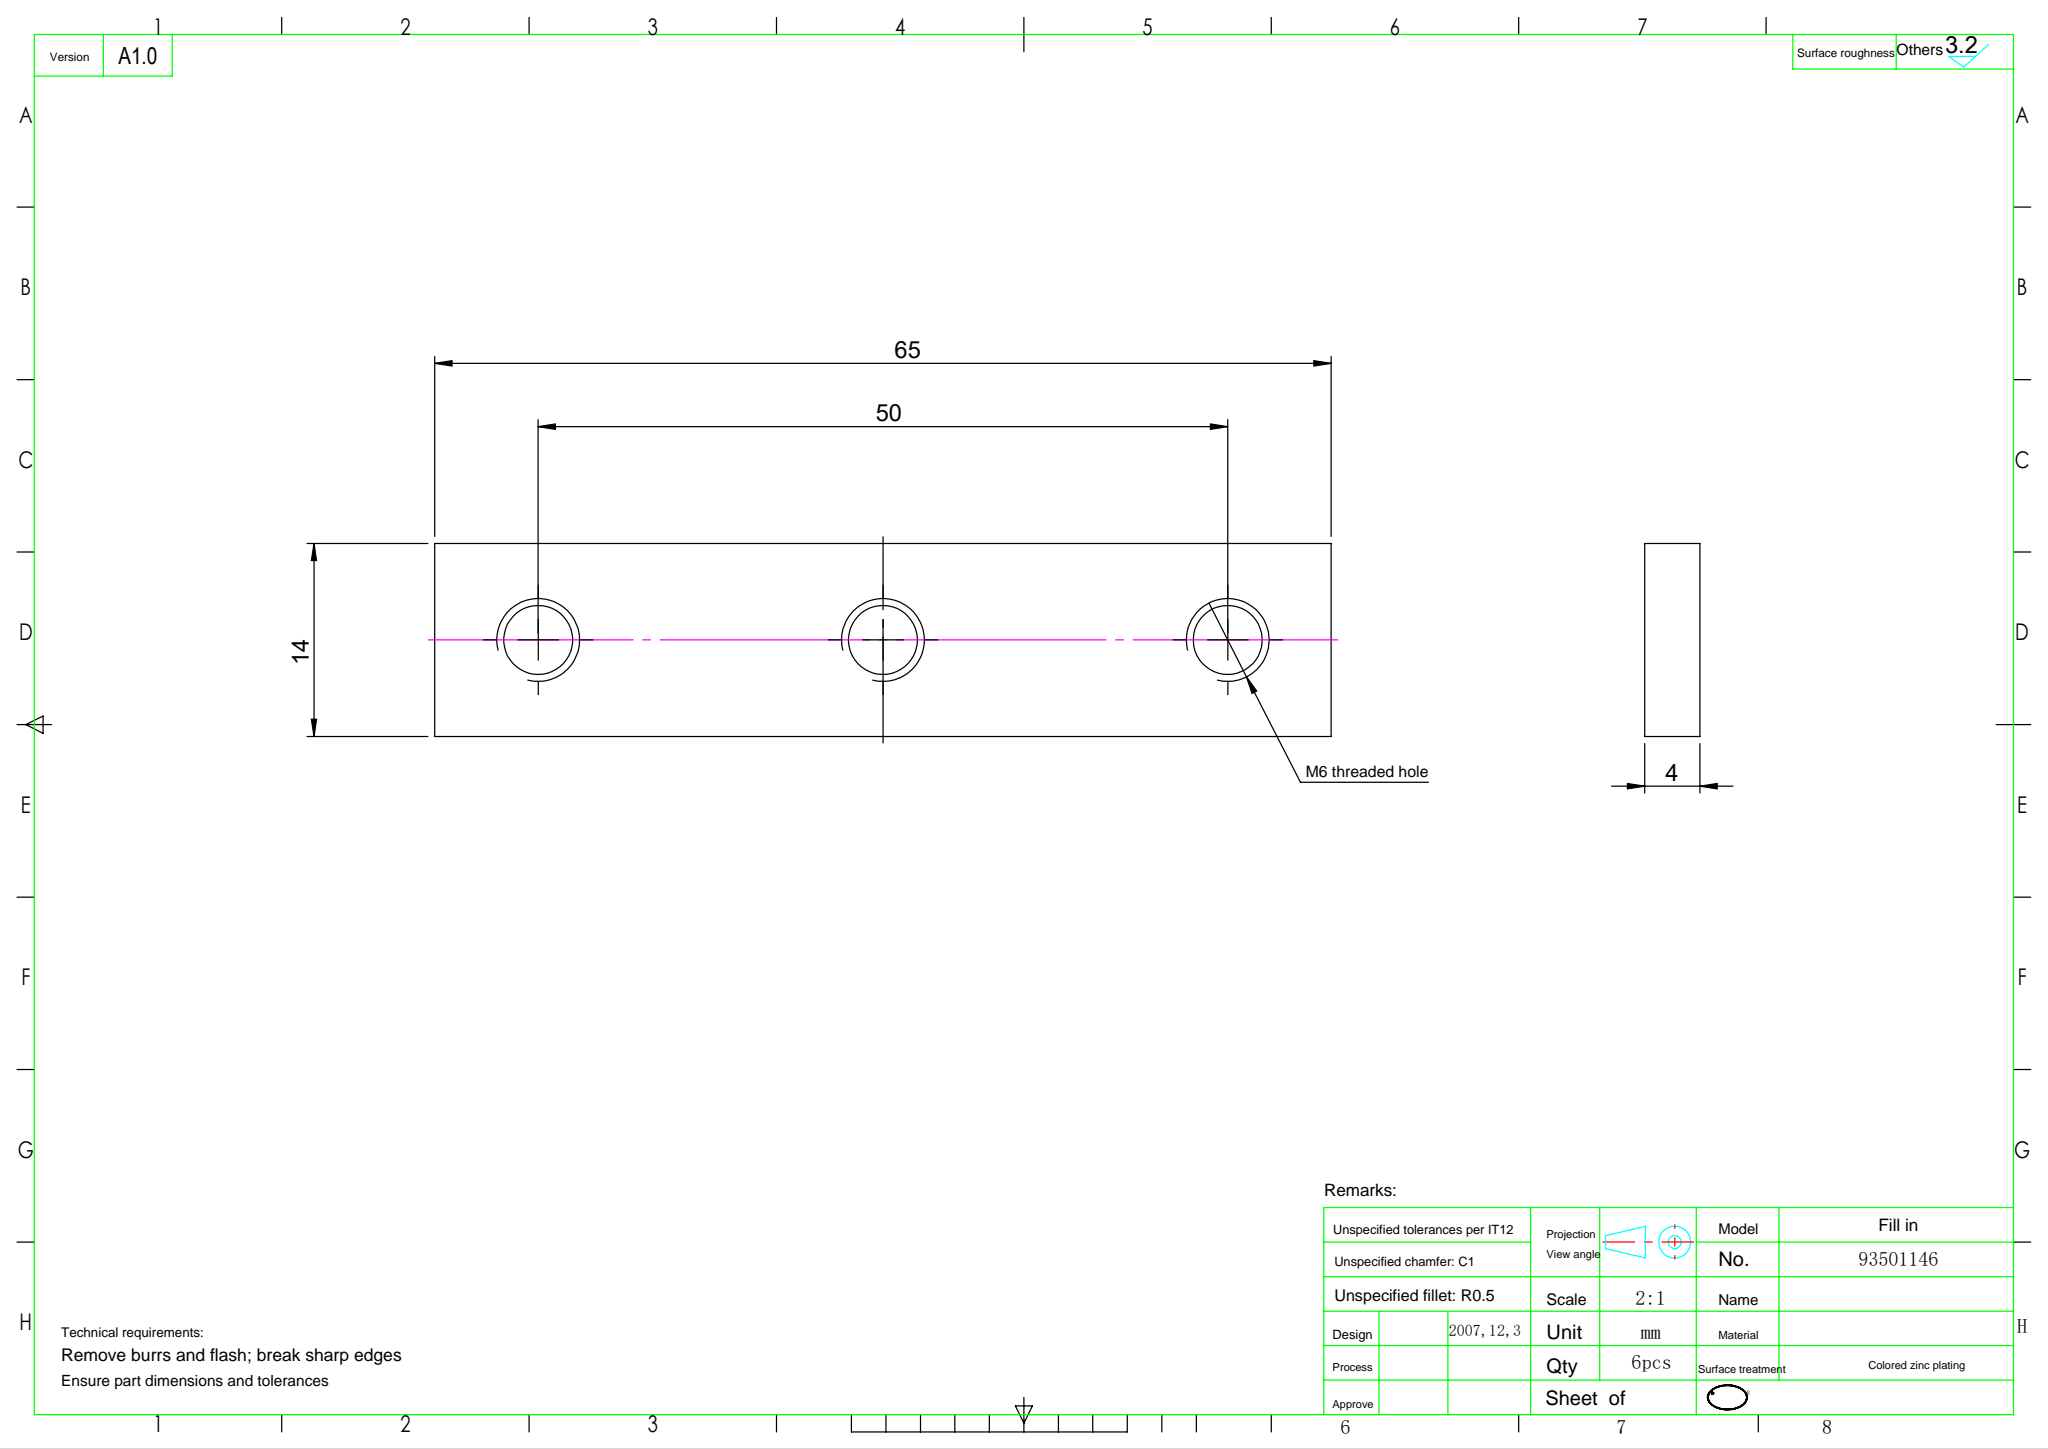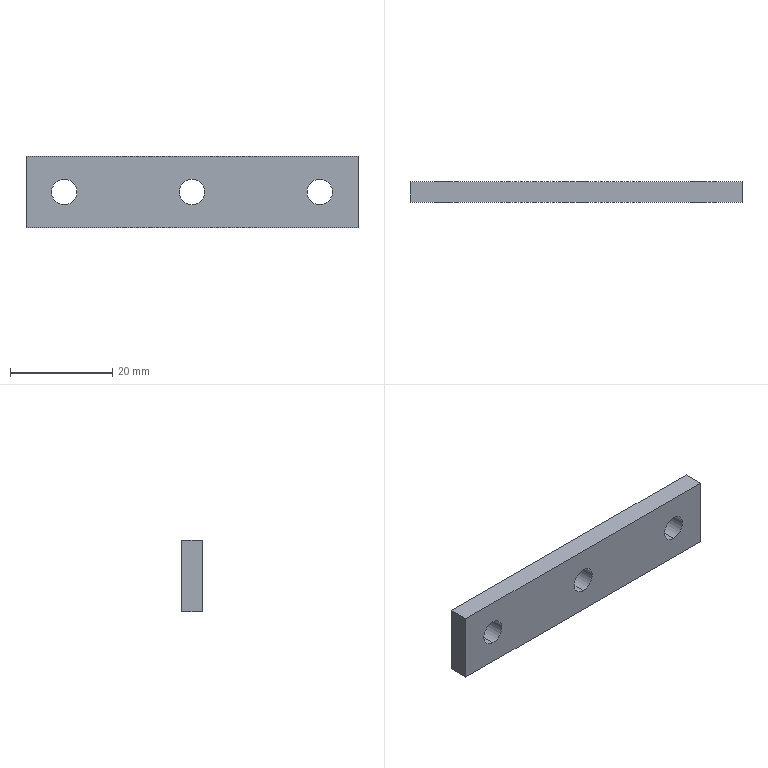Part | SolidWorks | features HoleWzd 1, ICE 1 | 1 solid | 12 faces | box 65 x 4 x 14 mm | volume 3404 mm3 | cylinder 6 | plane 6 | commonest cylinder face diameters 5 x6
STEP:
#1=CARTESIAN_POINT('',(-25.,-2.,-2.5));
#2=VERTEX_POINT('',#1);
#3=CARTESIAN_POINT('',(-25.,-2.,2.5));
#4=VERTEX_POINT('',#3);
#5=CARTESIAN_POINT('',(-25.,-2.,0.));
#6=DIRECTION('',(0.,1.,0.));
#7=DIRECTION('',(0.,0.,1.));
#8=AXIS2_PLACEMENT_3D('',#5,#6,#7);
#9=CIRCLE('',#8,2.5);
#10=EDGE_CURVE('',#2,#4,#9,.T.);
#11=ORIENTED_EDGE('',*,*,#10,.F.);
#12=CARTESIAN_POINT('',(-25.,2.,-2.5));
#13=VERTEX_POINT('',#12);
#14=CARTESIAN_POINT('',(-25.,2.,-2.5));
#15=DIRECTION('',(0.,1.,0.));
#16=VECTOR('',#15,1000.);
#17=LINE('',#14,#16);
#18=EDGE_CURVE('',#2,#13,#17,.T.);
#19=ORIENTED_EDGE('',*,*,#18,.T.);
#20=CARTESIAN_POINT('',(-25.,2.,2.5));
#21=VERTEX_POINT('',#20);
#22=CARTESIAN_POINT('',(-25.,2.,0.));
#23=DIRECTION('',(0.,1.,0.));
#24=DIRECTION('',(0.,0.,1.));
#25=AXIS2_PLACEMENT_3D('',#22,#23,#24);
#26=CIRCLE('',#25,2.5);
#27=EDGE_CURVE('',#13,#21,#26,.T.);
#28=ORIENTED_EDGE('',*,*,#27,.T.);
#29=CARTESIAN_POINT('',(-25.,2.,2.5));
#30=DIRECTION('',(0.,1.,0.));
#31=VECTOR('',#30,1000.);
#32=LINE('',#29,#31);
#33=EDGE_CURVE('',#4,#21,#32,.T.);
#34=ORIENTED_EDGE('',*,*,#33,.F.);
#35=EDGE_LOOP('',(#11,#19,#28,#34));
#36=FACE_OUTER_BOUND('',#35,.T.);
#37=CARTESIAN_POINT('',(-25.,2.,0.));
#38=DIRECTION('',(0.,1.,0.));
#39=DIRECTION('',(0.,0.,1.));
#40=AXIS2_PLACEMENT_3D('',#37,#38,#39);
#41=CYLINDRICAL_SURFACE('',#40,2.5);
#42=ADVANCED_FACE('',(#36),#41,.F.);
#43=CARTESIAN_POINT('',(0.,-2.,-2.5));
#44=VERTEX_POINT('',#43);
#45=CARTESIAN_POINT('',(0.,-2.,2.5));
#46=VERTEX_POINT('',#45);
#47=CARTESIAN_POINT('',(0.,-2.,0.));
#48=DIRECTION('',(0.,1.,0.));
#49=DIRECTION('',(0.,0.,1.));
#50=AXIS2_PLACEMENT_3D('',#47,#48,#49);
#51=CIRCLE('',#50,2.5);
#52=EDGE_CURVE('',#44,#46,#51,.T.);
#53=ORIENTED_EDGE('',*,*,#52,.F.);
#54=CARTESIAN_POINT('',(0.,2.,-2.5));
#55=VERTEX_POINT('',#54);
#56=CARTESIAN_POINT('',(0.,2.,-2.5));
#57=DIRECTION('',(0.,1.,0.));
#58=VECTOR('',#57,1000.);
#59=LINE('',#56,#58);
#60=EDGE_CURVE('',#44,#55,#59,.T.);
#61=ORIENTED_EDGE('',*,*,#60,.T.);
#62=CARTESIAN_POINT('',(0.,2.,2.5));
#63=VERTEX_POINT('',#62);
#64=CARTESIAN_POINT('',(0.,2.,0.));
#65=DIRECTION('',(0.,1.,0.));
#66=DIRECTION('',(0.,0.,1.));
#67=AXIS2_PLACEMENT_3D('',#64,#65,#66);
#68=CIRCLE('',#67,2.5);
#69=EDGE_CURVE('',#55,#63,#68,.T.);
#70=ORIENTED_EDGE('',*,*,#69,.T.);
#71=CARTESIAN_POINT('',(0.,2.,2.5));
#72=DIRECTION('',(0.,1.,0.));
#73=VECTOR('',#72,1000.);
#74=LINE('',#71,#73);
#75=EDGE_CURVE('',#46,#63,#74,.T.);
#76=ORIENTED_EDGE('',*,*,#75,.F.);
#77=EDGE_LOOP('',(#53,#61,#70,#76));
#78=FACE_OUTER_BOUND('',#77,.T.);
#79=CARTESIAN_POINT('',(0.,2.,0.));
#80=DIRECTION('',(0.,1.,0.));
#81=DIRECTION('',(0.,0.,1.));
#82=AXIS2_PLACEMENT_3D('',#79,#80,#81);
#83=CYLINDRICAL_SURFACE('',#82,2.5);
#84=ADVANCED_FACE('',(#78),#83,.F.);
#85=CARTESIAN_POINT('',(25.,-2.,-2.5));
#86=VERTEX_POINT('',#85);
#87=CARTESIAN_POINT('',(25.,-2.,2.5));
#88=VERTEX_POINT('',#87);
#89=CARTESIAN_POINT('',(25.,-2.,0.));
#90=DIRECTION('',(0.,1.,0.));
#91=DIRECTION('',(0.,0.,1.));
#92=AXIS2_PLACEMENT_3D('',#89,#90,#91);
#93=CIRCLE('',#92,2.5);
#94=EDGE_CURVE('',#86,#88,#93,.T.);
#95=ORIENTED_EDGE('',*,*,#94,.F.);
#96=CARTESIAN_POINT('',(25.,2.,-2.5));
#97=VERTEX_POINT('',#96);
#98=CARTESIAN_POINT('',(25.,2.,-2.5));
#99=DIRECTION('',(0.,1.,0.));
#100=VECTOR('',#99,1000.);
#101=LINE('',#98,#100);
#102=EDGE_CURVE('',#86,#97,#101,.T.);
#103=ORIENTED_EDGE('',*,*,#102,.T.);
#104=CARTESIAN_POINT('',(25.,2.,2.5));
#105=VERTEX_POINT('',#104);
#106=CARTESIAN_POINT('',(25.,2.,0.));
#107=DIRECTION('',(0.,1.,0.));
#108=DIRECTION('',(0.,0.,1.));
#109=AXIS2_PLACEMENT_3D('',#106,#107,#108);
#110=CIRCLE('',#109,2.5);
#111=EDGE_CURVE('',#97,#105,#110,.T.);
#112=ORIENTED_EDGE('',*,*,#111,.T.);
#113=CARTESIAN_POINT('',(25.,2.,2.5));
#114=DIRECTION('',(0.,1.,0.));
#115=VECTOR('',#114,1000.);
#116=LINE('',#113,#115);
#117=EDGE_CURVE('',#88,#105,#116,.T.);
#118=ORIENTED_EDGE('',*,*,#117,.F.);
#119=EDGE_LOOP('',(#95,#103,#112,#118));
#120=FACE_OUTER_BOUND('',#119,.T.);
#121=CARTESIAN_POINT('',(25.,2.,0.));
#122=DIRECTION('',(0.,1.,0.));
#123=DIRECTION('',(0.,0.,1.));
#124=AXIS2_PLACEMENT_3D('',#121,#122,#123);
#125=CYLINDRICAL_SURFACE('',#124,2.5);
#126=ADVANCED_FACE('',(#120),#125,.F.);
#127=CARTESIAN_POINT('',(32.5,-2.,7.));
#128=VERTEX_POINT('',#127);
#129=CARTESIAN_POINT('',(32.5,-2.,-7.));
#130=VERTEX_POINT('',#129);
#131=CARTESIAN_POINT('',(32.5,-2.,-7.));
#132=DIRECTION('',(0.,0.,-1.));
#133=VECTOR('',#132,1000.);
#134=LINE('',#131,#133);
#135=EDGE_CURVE('',#128,#130,#134,.T.);
#136=ORIENTED_EDGE('',*,*,#135,.T.);
#137=CARTESIAN_POINT('',(32.5,2.,-7.));
#138=VERTEX_POINT('',#137);
#139=CARTESIAN_POINT('',(32.5,2.,-7.));
#140=DIRECTION('',(0.,-1.,0.));
#141=VECTOR('',#140,1000.);
#142=LINE('',#139,#141);
#143=EDGE_CURVE('',#138,#130,#142,.T.);
#144=ORIENTED_EDGE('',*,*,#143,.F.);
#145=CARTESIAN_POINT('',(32.5,2.,7.));
#146=VERTEX_POINT('',#145);
#147=CARTESIAN_POINT('',(32.5,2.,-7.));
#148=DIRECTION('',(0.,0.,-1.));
#149=VECTOR('',#148,1000.);
#150=LINE('',#147,#149);
#151=EDGE_CURVE('',#146,#138,#150,.T.);
#152=ORIENTED_EDGE('',*,*,#151,.F.);
#153=CARTESIAN_POINT('',(32.5,2.,7.));
#154=DIRECTION('',(0.,-1.,0.));
#155=VECTOR('',#154,1000.);
#156=LINE('',#153,#155);
#157=EDGE_CURVE('',#146,#128,#156,.T.);
#158=ORIENTED_EDGE('',*,*,#157,.T.);
#159=EDGE_LOOP('',(#136,#144,#152,#158));
#160=FACE_OUTER_BOUND('',#159,.T.);
#161=CARTESIAN_POINT('',(32.5,2.,-7.));
#162=DIRECTION('',(-1.,0.,0.));
#163=DIRECTION('',(0.,0.,1.));
#164=AXIS2_PLACEMENT_3D('',#161,#162,#163);
#165=PLANE('',#164);
#166=ADVANCED_FACE('',(#160),#165,.F.);
#167=CARTESIAN_POINT('',(-32.5,-2.,-7.));
#168=VERTEX_POINT('',#167);
#169=CARTESIAN_POINT('',(-32.5,-2.,-7.));
#170=DIRECTION('',(-1.,0.,0.));
#171=VECTOR('',#170,1000.);
#172=LINE('',#169,#171);
#173=EDGE_CURVE('',#130,#168,#172,.T.);
#174=ORIENTED_EDGE('',*,*,#173,.T.);
#175=CARTESIAN_POINT('',(-32.5,2.,-7.));
#176=VERTEX_POINT('',#175);
#177=CARTESIAN_POINT('',(-32.5,2.,-7.));
#178=DIRECTION('',(0.,-1.,0.));
#179=VECTOR('',#178,1000.);
#180=LINE('',#177,#179);
#181=EDGE_CURVE('',#176,#168,#180,.T.);
#182=ORIENTED_EDGE('',*,*,#181,.F.);
#183=CARTESIAN_POINT('',(-32.5,2.,-7.));
#184=DIRECTION('',(-1.,0.,0.));
#185=VECTOR('',#184,1000.);
#186=LINE('',#183,#185);
#187=EDGE_CURVE('',#138,#176,#186,.T.);
#188=ORIENTED_EDGE('',*,*,#187,.F.);
#189=ORIENTED_EDGE('',*,*,#143,.T.);
#190=EDGE_LOOP('',(#174,#182,#188,#189));
#191=FACE_OUTER_BOUND('',#190,.T.);
#192=CARTESIAN_POINT('',(-32.5,2.,-7.));
#193=DIRECTION('',(0.,0.,1.));
#194=DIRECTION('',(1.,0.,0.));
#195=AXIS2_PLACEMENT_3D('',#192,#193,#194);
#196=PLANE('',#195);
#197=ADVANCED_FACE('',(#191),#196,.F.);
#198=CARTESIAN_POINT('',(-32.5,-2.,7.));
#199=VERTEX_POINT('',#198);
#200=CARTESIAN_POINT('',(-32.5,-2.,-7.));
#201=DIRECTION('',(0.,0.,1.));
#202=VECTOR('',#201,1000.);
#203=LINE('',#200,#202);
#204=EDGE_CURVE('',#168,#199,#203,.T.);
#205=ORIENTED_EDGE('',*,*,#204,.T.);
#206=CARTESIAN_POINT('',(-32.5,2.,7.));
#207=VERTEX_POINT('',#206);
#208=CARTESIAN_POINT('',(-32.5,2.,7.));
#209=DIRECTION('',(0.,-1.,0.));
#210=VECTOR('',#209,1000.);
#211=LINE('',#208,#210);
#212=EDGE_CURVE('',#207,#199,#211,.T.);
#213=ORIENTED_EDGE('',*,*,#212,.F.);
#214=CARTESIAN_POINT('',(-32.5,2.,-7.));
#215=DIRECTION('',(0.,0.,1.));
#216=VECTOR('',#215,1000.);
#217=LINE('',#214,#216);
#218=EDGE_CURVE('',#176,#207,#217,.T.);
#219=ORIENTED_EDGE('',*,*,#218,.F.);
#220=ORIENTED_EDGE('',*,*,#181,.T.);
#221=EDGE_LOOP('',(#205,#213,#219,#220));
#222=FACE_OUTER_BOUND('',#221,.T.);
#223=CARTESIAN_POINT('',(-32.5,2.,-7.));
#224=DIRECTION('',(1.,0.,0.));
#225=DIRECTION('',(0.,0.,-1.));
#226=AXIS2_PLACEMENT_3D('',#223,#224,#225);
#227=PLANE('',#226);
#228=ADVANCED_FACE('',(#222),#227,.F.);
#229=CARTESIAN_POINT('',(-32.5,-2.,7.));
#230=DIRECTION('',(1.,0.,0.));
#231=VECTOR('',#230,1000.);
#232=LINE('',#229,#231);
#233=EDGE_CURVE('',#199,#128,#232,.T.);
#234=ORIENTED_EDGE('',*,*,#233,.T.);
#235=ORIENTED_EDGE('',*,*,#157,.F.);
#236=CARTESIAN_POINT('',(-32.5,2.,7.));
#237=DIRECTION('',(1.,0.,0.));
#238=VECTOR('',#237,1000.);
#239=LINE('',#236,#238);
#240=EDGE_CURVE('',#207,#146,#239,.T.);
#241=ORIENTED_EDGE('',*,*,#240,.F.);
#242=ORIENTED_EDGE('',*,*,#212,.T.);
#243=EDGE_LOOP('',(#234,#235,#241,#242));
#244=FACE_OUTER_BOUND('',#243,.T.);
#245=CARTESIAN_POINT('',(-32.5,2.,7.));
#246=DIRECTION('',(0.,0.,-1.));
#247=DIRECTION('',(-1.,0.,0.));
#248=AXIS2_PLACEMENT_3D('',#245,#246,#247);
#249=PLANE('',#248);
#250=ADVANCED_FACE('',(#244),#249,.F.);
#251=CARTESIAN_POINT('',(-25.,2.,0.));
#252=DIRECTION('',(0.,1.,0.));
#253=DIRECTION('',(0.,0.,1.));
#254=AXIS2_PLACEMENT_3D('',#251,#252,#253);
#255=CIRCLE('',#254,2.5);
#256=EDGE_CURVE('',#21,#13,#255,.T.);
#257=ORIENTED_EDGE('',*,*,#256,.F.);
#258=ORIENTED_EDGE('',*,*,#27,.F.);
#259=EDGE_LOOP('',(#257,#258));
#260=FACE_BOUND('',#259,.T.);
#261=CARTESIAN_POINT('',(0.,2.,0.));
#262=DIRECTION('',(0.,1.,0.));
#263=DIRECTION('',(0.,0.,1.));
#264=AXIS2_PLACEMENT_3D('',#261,#262,#263);
#265=CIRCLE('',#264,2.5);
#266=EDGE_CURVE('',#63,#55,#265,.T.);
#267=ORIENTED_EDGE('',*,*,#266,.F.);
#268=ORIENTED_EDGE('',*,*,#69,.F.);
#269=EDGE_LOOP('',(#267,#268));
#270=FACE_BOUND('',#269,.T.);
#271=CARTESIAN_POINT('',(25.,2.,0.));
#272=DIRECTION('',(0.,1.,0.));
#273=DIRECTION('',(0.,0.,1.));
#274=AXIS2_PLACEMENT_3D('',#271,#272,#273);
#275=CIRCLE('',#274,2.5);
#276=EDGE_CURVE('',#105,#97,#275,.T.);
#277=ORIENTED_EDGE('',*,*,#276,.F.);
#278=ORIENTED_EDGE('',*,*,#111,.F.);
#279=EDGE_LOOP('',(#277,#278));
#280=FACE_BOUND('',#279,.T.);
#281=ORIENTED_EDGE('',*,*,#151,.T.);
#282=ORIENTED_EDGE('',*,*,#187,.T.);
#283=ORIENTED_EDGE('',*,*,#218,.T.);
#284=ORIENTED_EDGE('',*,*,#240,.T.);
#285=EDGE_LOOP('',(#281,#282,#283,#284));
#286=FACE_OUTER_BOUND('',#285,.T.);
#287=CARTESIAN_POINT('',(0.,2.,0.));
#288=DIRECTION('',(0.,1.,0.));
#289=DIRECTION('',(0.,0.,1.));
#290=AXIS2_PLACEMENT_3D('',#287,#288,#289);
#291=PLANE('',#290);
#292=ADVANCED_FACE('',(#260,#270,#280,#286),#291,.T.);
#293=CARTESIAN_POINT('',(-25.,-2.,0.));
#294=DIRECTION('',(0.,1.,0.));
#295=DIRECTION('',(0.,0.,1.));
#296=AXIS2_PLACEMENT_3D('',#293,#294,#295);
#297=CIRCLE('',#296,2.5);
#298=EDGE_CURVE('',#4,#2,#297,.T.);
#299=ORIENTED_EDGE('',*,*,#298,.T.);
#300=ORIENTED_EDGE('',*,*,#10,.T.);
#301=EDGE_LOOP('',(#299,#300));
#302=FACE_BOUND('',#301,.T.);
#303=CARTESIAN_POINT('',(0.,-2.,0.));
#304=DIRECTION('',(0.,1.,0.));
#305=DIRECTION('',(0.,0.,1.));
#306=AXIS2_PLACEMENT_3D('',#303,#304,#305);
#307=CIRCLE('',#306,2.5);
#308=EDGE_CURVE('',#46,#44,#307,.T.);
#309=ORIENTED_EDGE('',*,*,#308,.T.);
#310=ORIENTED_EDGE('',*,*,#52,.T.);
#311=EDGE_LOOP('',(#309,#310));
#312=FACE_BOUND('',#311,.T.);
#313=CARTESIAN_POINT('',(25.,-2.,0.));
#314=DIRECTION('',(0.,1.,0.));
#315=DIRECTION('',(0.,0.,1.));
#316=AXIS2_PLACEMENT_3D('',#313,#314,#315);
#317=CIRCLE('',#316,2.5);
#318=EDGE_CURVE('',#88,#86,#317,.T.);
#319=ORIENTED_EDGE('',*,*,#318,.T.);
#320=ORIENTED_EDGE('',*,*,#94,.T.);
#321=EDGE_LOOP('',(#319,#320));
#322=FACE_BOUND('',#321,.T.);
#323=ORIENTED_EDGE('',*,*,#135,.F.);
#324=ORIENTED_EDGE('',*,*,#233,.F.);
#325=ORIENTED_EDGE('',*,*,#204,.F.);
#326=ORIENTED_EDGE('',*,*,#173,.F.);
#327=EDGE_LOOP('',(#323,#324,#325,#326));
#328=FACE_OUTER_BOUND('',#327,.T.);
#329=CARTESIAN_POINT('',(0.,-2.,0.));
#330=DIRECTION('',(0.,1.,0.));
#331=DIRECTION('',(0.,0.,1.));
#332=AXIS2_PLACEMENT_3D('',#329,#330,#331);
#333=PLANE('',#332);
#334=ADVANCED_FACE('',(#302,#312,#322,#328),#333,.F.);
#335=ORIENTED_EDGE('',*,*,#102,.F.);
#336=ORIENTED_EDGE('',*,*,#318,.F.);
#337=ORIENTED_EDGE('',*,*,#117,.T.);
#338=ORIENTED_EDGE('',*,*,#276,.T.);
#339=EDGE_LOOP('',(#335,#336,#337,#338));
#340=FACE_OUTER_BOUND('',#339,.T.);
#341=CARTESIAN_POINT('',(25.,2.,0.));
#342=DIRECTION('',(0.,1.,0.));
#343=DIRECTION('',(0.,0.,1.));
#344=AXIS2_PLACEMENT_3D('',#341,#342,#343);
#345=CYLINDRICAL_SURFACE('',#344,2.5);
#346=ADVANCED_FACE('',(#340),#345,.F.);
#347=ORIENTED_EDGE('',*,*,#60,.F.);
#348=ORIENTED_EDGE('',*,*,#308,.F.);
#349=ORIENTED_EDGE('',*,*,#75,.T.);
#350=ORIENTED_EDGE('',*,*,#266,.T.);
#351=EDGE_LOOP('',(#347,#348,#349,#350));
#352=FACE_OUTER_BOUND('',#351,.T.);
#353=CARTESIAN_POINT('',(0.,2.,0.));
#354=DIRECTION('',(0.,1.,0.));
#355=DIRECTION('',(0.,0.,1.));
#356=AXIS2_PLACEMENT_3D('',#353,#354,#355);
#357=CYLINDRICAL_SURFACE('',#356,2.5);
#358=ADVANCED_FACE('',(#352),#357,.F.);
#359=ORIENTED_EDGE('',*,*,#18,.F.);
#360=ORIENTED_EDGE('',*,*,#298,.F.);
#361=ORIENTED_EDGE('',*,*,#33,.T.);
#362=ORIENTED_EDGE('',*,*,#256,.T.);
#363=EDGE_LOOP('',(#359,#360,#361,#362));
#364=FACE_OUTER_BOUND('',#363,.T.);
#365=CARTESIAN_POINT('',(-25.,2.,0.));
#366=DIRECTION('',(0.,1.,0.));
#367=DIRECTION('',(0.,0.,1.));
#368=AXIS2_PLACEMENT_3D('',#365,#366,#367);
#369=CYLINDRICAL_SURFACE('',#368,2.5);
#370=ADVANCED_FACE('',(#364),#369,.F.);
#371=CLOSED_SHELL('',(#42,#84,#126,#166,#197,#228,#250,#292,#334,#346,#358,#370));
#372=MANIFOLD_SOLID_BREP('',#371);
#373=CARTESIAN_POINT('',(0.,0.,0.));
#374=DIRECTION('',(0.,0.,1.));
#375=DIRECTION('',(1.,0.,0.));
#376=AXIS2_PLACEMENT_3D('',#373,#374,#375);
#377=(LENGTH_UNIT()NAMED_UNIT(*)SI_UNIT(.MILLI.,.METRE.));
#378=UNCERTAINTY_MEASURE_WITH_UNIT(LENGTH_MEASURE(0.00001),#377,'','');
#379=(NAMED_UNIT(*)PLANE_ANGLE_UNIT()SI_UNIT($,.RADIAN.));
#380=(NAMED_UNIT(*)SI_UNIT($,.STERADIAN.)SOLID_ANGLE_UNIT());
#381=(GEOMETRIC_REPRESENTATION_CONTEXT(3)GLOBAL_UNCERTAINTY_ASSIGNED_CONTEXT((#378))GLOBAL_UNIT_ASSIGNED_CONTEXT((#377,#379,#380))REPRESENTATION_CONTEXT('',''));
#382=ADVANCED_BREP_SHAPE_REPRESENTATION('',(#372,#376),#381);